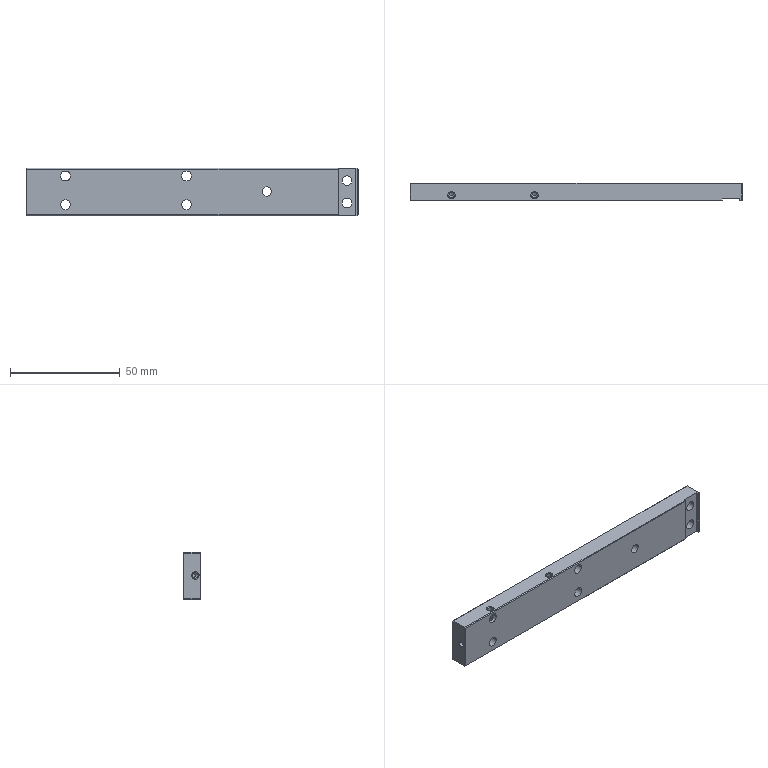Part | NX | 1 solid | 77 faces | box 151 x 8 x 21.5 mm | volume 24803 mm3 | cylinder 28 | cone 26 | plane 23 | commonest cylinder face diameters 2.5 x14 4.5 x12 4.2 x2